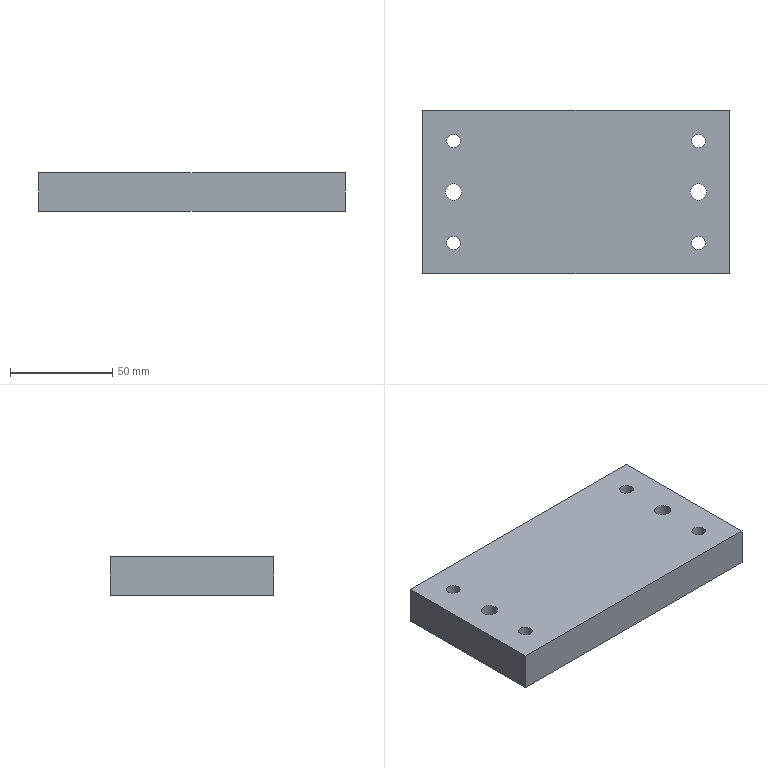Part | STEP file | SN10_010_005-01_PLACA | 1 solid | 12 faces | box 150 x 80 x 19 mm | volume 223453 mm3 | cylinder 6 | plane 6 | commonest cylinder face diameters 6.647 x4 8 x2
STEP:
#1=CARTESIAN_POINT('',(0.,0.,0.));
#2=DIRECTION('',(0.,0.,1.));
#3=DIRECTION('',(1.,0.,0.));
#4=AXIS2_PLACEMENT_3D('',#1,#2,#3);
#5=CARTESIAN_POINT('',(-57.083,-286.593,339.));
#6=VERTEX_POINT('',#5);
#7=CARTESIAN_POINT('',(-60.,-285.,339.));
#8=DIRECTION('',(0.,0.,-1.));
#9=DIRECTION('',(1.,0.,0.));
#10=AXIS2_PLACEMENT_3D('',#7,#8,#9);
#11=CIRCLE('',#10,3.324);
#12=CARTESIAN_POINT('',(-60.,-285.,338.9));
#13=DIRECTION('',(0.,0.,-1.));
#14=DIRECTION('',(0.8776,-0.4794,0.));
#15=AXIS2_PLACEMENT_3D('',#12,#13,#14);
#16=CYLINDRICAL_SURFACE('',#15,3.324);
#17=CARTESIAN_POINT('',(-0.5,-0.1));
#18=DIRECTION('',(1.,0.));
#19=VECTOR('',#18,1.);
#20=LINE('',#17,#19);
#21=(GEOMETRIC_REPRESENTATION_CONTEXT(2)PARAMETRIC_REPRESENTATION_CONTEXT()REPRESENTATION_CONTEXT('',''));
#22=DEFINITIONAL_REPRESENTATION('',(#20),#21);
#23=PCURVE('',#16,#22);
#24=CARTESIAN_POINT('',(0.,0.,339.));
#25=DIRECTION('',(0.,0.,1.));
#26=DIRECTION('',(1.,0.,0.));
#27=AXIS2_PLACEMENT_3D('',#24,#25,#26);
#28=PLANE('',#27);
#29=CARTESIAN_POINT('',(-56.676,-285.));
#30=CARTESIAN_POINT('',(-56.676,-290.756));
#31=CARTESIAN_POINT('',(-61.662,-287.878));
#32=CARTESIAN_POINT('',(-66.647,-285.));
#33=CARTESIAN_POINT('',(-61.662,-282.122));
#34=CARTESIAN_POINT('',(-56.676,-279.244));
#35=CARTESIAN_POINT('',(-56.676,-285.));
#36=(BOUNDED_CURVE()B_SPLINE_CURVE(2,(#29,#30,#31,#32,#33,#34,#35),.UNSPECIFIED.,.T.,.F.)B_SPLINE_CURVE_WITH_KNOTS((1,2,2,2,2,1),(-2.094,0.,2.094,4.189,6.283,8.378),.UNSPECIFIED.)CURVE()GEOMETRIC_REPRESENTATION_ITEM()RATIONAL_B_SPLINE_CURVE((1.,0.5,1.,0.5,1.,0.5,1.))REPRESENTATION_ITEM(''));
#37=(GEOMETRIC_REPRESENTATION_CONTEXT(2)PARAMETRIC_REPRESENTATION_CONTEXT()REPRESENTATION_CONTEXT('',''));
#38=DEFINITIONAL_REPRESENTATION('',(#36),#37);
#39=PCURVE('',#28,#38);
#40=SURFACE_CURVE('',#11,(#23,#39),.PCURVE_S1.);
#41=EDGE_CURVE('',#6,#6,#40,.T.);
#42=ORIENTED_EDGE('',*,*,#41,.T.);
#43=CARTESIAN_POINT('',(-57.083,-286.593,320.));
#44=VERTEX_POINT('',#43);
#45=CARTESIAN_POINT('',(-57.083,-286.593,339.));
#46=CARTESIAN_POINT('',(-57.083,-286.593,320.));
#47=B_SPLINE_CURVE_WITH_KNOTS('',1,(#45,#46),.UNSPECIFIED.,.F.,.F.,(2,2),(-0.1,18.9),.PIECEWISE_BEZIER_KNOTS.);
#48=CARTESIAN_POINT('',(6.283,0.));
#49=DIRECTION('',(0.,1.));
#50=VECTOR('',#49,1.);
#51=LINE('',#48,#50);
#52=(GEOMETRIC_REPRESENTATION_CONTEXT(2)PARAMETRIC_REPRESENTATION_CONTEXT()REPRESENTATION_CONTEXT('',''));
#53=DEFINITIONAL_REPRESENTATION('',(#51),#52);
#54=PCURVE('',#16,#53);
#55=CARTESIAN_POINT('',(0.,0.));
#56=DIRECTION('',(0.,1.));
#57=VECTOR('',#56,1.);
#58=LINE('',#55,#57);
#59=(GEOMETRIC_REPRESENTATION_CONTEXT(2)PARAMETRIC_REPRESENTATION_CONTEXT()REPRESENTATION_CONTEXT('',''));
#60=DEFINITIONAL_REPRESENTATION('',(#58),#59);
#61=PCURVE('',#16,#60);
#62=SEAM_CURVE('',#47,(#54,#61),.PCURVE_S1.);
#63=EDGE_CURVE('',#6,#44,#62,.T.);
#64=ORIENTED_EDGE('',*,*,#63,.T.);
#65=CARTESIAN_POINT('',(-60.,-285.,320.));
#66=DIRECTION('',(0.,0.,-1.));
#67=DIRECTION('',(1.,0.,0.));
#68=AXIS2_PLACEMENT_3D('',#65,#66,#67);
#69=CIRCLE('',#68,3.324);
#70=CARTESIAN_POINT('',(-0.5,18.9));
#71=DIRECTION('',(1.,0.));
#72=VECTOR('',#71,1.);
#73=LINE('',#70,#72);
#74=(GEOMETRIC_REPRESENTATION_CONTEXT(2)PARAMETRIC_REPRESENTATION_CONTEXT()REPRESENTATION_CONTEXT('',''));
#75=DEFINITIONAL_REPRESENTATION('',(#73),#74);
#76=PCURVE('',#16,#75);
#77=CARTESIAN_POINT('',(0.,0.,320.));
#78=DIRECTION('',(0.,0.,1.));
#79=DIRECTION('',(1.,0.,0.));
#80=AXIS2_PLACEMENT_3D('',#77,#78,#79);
#81=PLANE('',#80);
#82=CARTESIAN_POINT('',(-56.676,-285.));
#83=CARTESIAN_POINT('',(-56.676,-290.756));
#84=CARTESIAN_POINT('',(-61.662,-287.878));
#85=CARTESIAN_POINT('',(-66.647,-285.));
#86=CARTESIAN_POINT('',(-61.662,-282.122));
#87=CARTESIAN_POINT('',(-56.676,-279.244));
#88=CARTESIAN_POINT('',(-56.676,-285.));
#89=(BOUNDED_CURVE()B_SPLINE_CURVE(2,(#82,#83,#84,#85,#86,#87,#88),.UNSPECIFIED.,.T.,.F.)B_SPLINE_CURVE_WITH_KNOTS((1,2,2,2,2,1),(-2.094,0.,2.094,4.189,6.283,8.378),.UNSPECIFIED.)CURVE()GEOMETRIC_REPRESENTATION_ITEM()RATIONAL_B_SPLINE_CURVE((1.,0.5,1.,0.5,1.,0.5,1.))REPRESENTATION_ITEM(''));
#90=(GEOMETRIC_REPRESENTATION_CONTEXT(2)PARAMETRIC_REPRESENTATION_CONTEXT()REPRESENTATION_CONTEXT('',''));
#91=DEFINITIONAL_REPRESENTATION('',(#89),#90);
#92=PCURVE('',#81,#91);
#93=SURFACE_CURVE('',#69,(#76,#92),.PCURVE_S1.);
#94=EDGE_CURVE('',#44,#44,#93,.T.);
#95=ORIENTED_EDGE('',*,*,#94,.F.);
#96=ORIENTED_EDGE('',*,*,#63,.F.);
#97=EDGE_LOOP('',(#42,#64,#95,#96));
#98=FACE_BOUND('',#97,.F.);
#99=ADVANCED_FACE('',(#98),#16,.F.);
#100=CARTESIAN_POINT('',(-75.,-270.,320.));
#101=VERTEX_POINT('',#100);
#102=CARTESIAN_POINT('',(-75.,-270.,339.));
#103=VERTEX_POINT('',#102);
#104=CARTESIAN_POINT('',(-75.,-270.,320.));
#105=DIRECTION('',(0.,0.,1.));
#106=VECTOR('',#105,1.);
#107=LINE('',#104,#106);
#108=CARTESIAN_POINT('',(-75.,-270.,320.));
#109=DIRECTION('',(-1.,0.,0.));
#110=DIRECTION('',(0.,0.,1.));
#111=AXIS2_PLACEMENT_3D('',#108,#109,#110);
#112=PLANE('',#111);
#113=CARTESIAN_POINT('',(0.,0.));
#114=DIRECTION('',(1.,0.));
#115=VECTOR('',#114,1.);
#116=LINE('',#113,#115);
#117=(GEOMETRIC_REPRESENTATION_CONTEXT(2)PARAMETRIC_REPRESENTATION_CONTEXT()REPRESENTATION_CONTEXT('',''));
#118=DEFINITIONAL_REPRESENTATION('',(#116),#117);
#119=PCURVE('',#112,#118);
#120=CARTESIAN_POINT('',(-75.,-270.,320.));
#121=DIRECTION('',(0.,-1.,0.));
#122=DIRECTION('',(0.,0.,-1.));
#123=AXIS2_PLACEMENT_3D('',#120,#121,#122);
#124=PLANE('',#123);
#125=CARTESIAN_POINT('',(0.,0.));
#126=DIRECTION('',(-1.,0.));
#127=VECTOR('',#126,1.);
#128=LINE('',#125,#127);
#129=(GEOMETRIC_REPRESENTATION_CONTEXT(2)PARAMETRIC_REPRESENTATION_CONTEXT()REPRESENTATION_CONTEXT('',''));
#130=DEFINITIONAL_REPRESENTATION('',(#128),#129);
#131=PCURVE('',#124,#130);
#132=SURFACE_CURVE('',#107,(#119,#131),.PCURVE_S1.);
#133=EDGE_CURVE('',#101,#103,#132,.T.);
#134=ORIENTED_EDGE('',*,*,#133,.F.);
#135=CARTESIAN_POINT('',(-75.,-350.,320.));
#136=VERTEX_POINT('',#135);
#137=CARTESIAN_POINT('',(-75.,-270.,320.));
#138=DIRECTION('',(0.,-1.,0.));
#139=VECTOR('',#138,1.);
#140=LINE('',#137,#139);
#141=CARTESIAN_POINT('',(0.,0.));
#142=DIRECTION('',(0.,-1.));
#143=VECTOR('',#142,1.);
#144=LINE('',#141,#143);
#145=(GEOMETRIC_REPRESENTATION_CONTEXT(2)PARAMETRIC_REPRESENTATION_CONTEXT()REPRESENTATION_CONTEXT('',''));
#146=DEFINITIONAL_REPRESENTATION('',(#144),#145);
#147=PCURVE('',#112,#146);
#148=CARTESIAN_POINT('',(-75.,-270.));
#149=DIRECTION('',(0.,-1.));
#150=VECTOR('',#149,1.);
#151=LINE('',#148,#150);
#152=(GEOMETRIC_REPRESENTATION_CONTEXT(2)PARAMETRIC_REPRESENTATION_CONTEXT()REPRESENTATION_CONTEXT('',''));
#153=DEFINITIONAL_REPRESENTATION('',(#151),#152);
#154=PCURVE('',#81,#153);
#155=SURFACE_CURVE('',#140,(#147,#154),.PCURVE_S1.);
#156=EDGE_CURVE('',#101,#136,#155,.T.);
#157=ORIENTED_EDGE('',*,*,#156,.T.);
#158=CARTESIAN_POINT('',(-75.,-350.,339.));
#159=VERTEX_POINT('',#158);
#160=CARTESIAN_POINT('',(-75.,-350.,320.));
#161=DIRECTION('',(0.,0.,1.));
#162=VECTOR('',#161,1.);
#163=LINE('',#160,#162);
#164=CARTESIAN_POINT('',(0.,-80.));
#165=DIRECTION('',(1.,0.));
#166=VECTOR('',#165,1.);
#167=LINE('',#164,#166);
#168=(GEOMETRIC_REPRESENTATION_CONTEXT(2)PARAMETRIC_REPRESENTATION_CONTEXT()REPRESENTATION_CONTEXT('',''));
#169=DEFINITIONAL_REPRESENTATION('',(#167),#168);
#170=PCURVE('',#112,#169);
#171=CARTESIAN_POINT('',(75.,-350.,320.));
#172=DIRECTION('',(0.,1.,0.));
#173=DIRECTION('',(0.,0.,1.));
#174=AXIS2_PLACEMENT_3D('',#171,#172,#173);
#175=PLANE('',#174);
#176=CARTESIAN_POINT('',(0.,-150.));
#177=DIRECTION('',(1.,0.));
#178=VECTOR('',#177,1.);
#179=LINE('',#176,#178);
#180=(GEOMETRIC_REPRESENTATION_CONTEXT(2)PARAMETRIC_REPRESENTATION_CONTEXT()REPRESENTATION_CONTEXT('',''));
#181=DEFINITIONAL_REPRESENTATION('',(#179),#180);
#182=PCURVE('',#175,#181);
#183=SURFACE_CURVE('',#163,(#170,#182),.PCURVE_S1.);
#184=EDGE_CURVE('',#136,#159,#183,.T.);
#185=ORIENTED_EDGE('',*,*,#184,.T.);
#186=CARTESIAN_POINT('',(-75.,-270.,339.));
#187=DIRECTION('',(0.,-1.,0.));
#188=VECTOR('',#187,1.);
#189=LINE('',#186,#188);
#190=CARTESIAN_POINT('',(19.,0.));
#191=DIRECTION('',(0.,-1.));
#192=VECTOR('',#191,1.);
#193=LINE('',#190,#192);
#194=(GEOMETRIC_REPRESENTATION_CONTEXT(2)PARAMETRIC_REPRESENTATION_CONTEXT()REPRESENTATION_CONTEXT('',''));
#195=DEFINITIONAL_REPRESENTATION('',(#193),#194);
#196=PCURVE('',#112,#195);
#197=CARTESIAN_POINT('',(-75.,-270.));
#198=DIRECTION('',(0.,-1.));
#199=VECTOR('',#198,1.);
#200=LINE('',#197,#199);
#201=(GEOMETRIC_REPRESENTATION_CONTEXT(2)PARAMETRIC_REPRESENTATION_CONTEXT()REPRESENTATION_CONTEXT('',''));
#202=DEFINITIONAL_REPRESENTATION('',(#200),#201);
#203=PCURVE('',#28,#202);
#204=SURFACE_CURVE('',#189,(#196,#203),.PCURVE_S1.);
#205=EDGE_CURVE('',#103,#159,#204,.T.);
#206=ORIENTED_EDGE('',*,*,#205,.F.);
#207=EDGE_LOOP('',(#134,#157,#185,#206));
#208=FACE_BOUND('',#207,.T.);
#209=ADVANCED_FACE('',(#208),#112,.T.);
#210=ORIENTED_EDGE('',*,*,#184,.F.);
#211=CARTESIAN_POINT('',(75.,-350.,320.));
#212=VERTEX_POINT('',#211);
#213=CARTESIAN_POINT('',(75.,-350.,320.));
#214=DIRECTION('',(-1.,0.,0.));
#215=VECTOR('',#214,1.);
#216=LINE('',#213,#215);
#217=CARTESIAN_POINT('',(0.,0.));
#218=DIRECTION('',(0.,-1.));
#219=VECTOR('',#218,1.);
#220=LINE('',#217,#219);
#221=(GEOMETRIC_REPRESENTATION_CONTEXT(2)PARAMETRIC_REPRESENTATION_CONTEXT()REPRESENTATION_CONTEXT('',''));
#222=DEFINITIONAL_REPRESENTATION('',(#220),#221);
#223=PCURVE('',#175,#222);
#224=CARTESIAN_POINT('',(75.,-350.));
#225=DIRECTION('',(-1.,0.));
#226=VECTOR('',#225,1.);
#227=LINE('',#224,#226);
#228=(GEOMETRIC_REPRESENTATION_CONTEXT(2)PARAMETRIC_REPRESENTATION_CONTEXT()REPRESENTATION_CONTEXT('',''));
#229=DEFINITIONAL_REPRESENTATION('',(#227),#228);
#230=PCURVE('',#81,#229);
#231=SURFACE_CURVE('',#216,(#223,#230),.PCURVE_S1.);
#232=EDGE_CURVE('',#212,#136,#231,.T.);
#233=ORIENTED_EDGE('',*,*,#232,.F.);
#234=CARTESIAN_POINT('',(75.,-350.,339.));
#235=VERTEX_POINT('',#234);
#236=CARTESIAN_POINT('',(75.,-350.,320.));
#237=DIRECTION('',(0.,0.,1.));
#238=VECTOR('',#237,1.);
#239=LINE('',#236,#238);
#240=CARTESIAN_POINT('',(0.,0.));
#241=DIRECTION('',(1.,0.));
#242=VECTOR('',#241,1.);
#243=LINE('',#240,#242);
#244=(GEOMETRIC_REPRESENTATION_CONTEXT(2)PARAMETRIC_REPRESENTATION_CONTEXT()REPRESENTATION_CONTEXT('',''));
#245=DEFINITIONAL_REPRESENTATION('',(#243),#244);
#246=PCURVE('',#175,#245);
#247=CARTESIAN_POINT('',(75.,-350.,320.));
#248=DIRECTION('',(1.,0.,0.));
#249=DIRECTION('',(0.,0.,-1.));
#250=AXIS2_PLACEMENT_3D('',#247,#248,#249);
#251=PLANE('',#250);
#252=CARTESIAN_POINT('',(0.,0.));
#253=DIRECTION('',(-1.,0.));
#254=VECTOR('',#253,1.);
#255=LINE('',#252,#254);
#256=(GEOMETRIC_REPRESENTATION_CONTEXT(2)PARAMETRIC_REPRESENTATION_CONTEXT()REPRESENTATION_CONTEXT('',''));
#257=DEFINITIONAL_REPRESENTATION('',(#255),#256);
#258=PCURVE('',#251,#257);
#259=SURFACE_CURVE('',#239,(#246,#258),.PCURVE_S1.);
#260=EDGE_CURVE('',#212,#235,#259,.T.);
#261=ORIENTED_EDGE('',*,*,#260,.T.);
#262=CARTESIAN_POINT('',(75.,-350.,339.));
#263=DIRECTION('',(-1.,0.,0.));
#264=VECTOR('',#263,1.);
#265=LINE('',#262,#264);
#266=CARTESIAN_POINT('',(19.,0.));
#267=DIRECTION('',(0.,-1.));
#268=VECTOR('',#267,1.);
#269=LINE('',#266,#268);
#270=(GEOMETRIC_REPRESENTATION_CONTEXT(2)PARAMETRIC_REPRESENTATION_CONTEXT()REPRESENTATION_CONTEXT('',''));
#271=DEFINITIONAL_REPRESENTATION('',(#269),#270);
#272=PCURVE('',#175,#271);
#273=CARTESIAN_POINT('',(75.,-350.));
#274=DIRECTION('',(-1.,0.));
#275=VECTOR('',#274,1.);
#276=LINE('',#273,#275);
#277=(GEOMETRIC_REPRESENTATION_CONTEXT(2)PARAMETRIC_REPRESENTATION_CONTEXT()REPRESENTATION_CONTEXT('',''));
#278=DEFINITIONAL_REPRESENTATION('',(#276),#277);
#279=PCURVE('',#28,#278);
#280=SURFACE_CURVE('',#265,(#272,#279),.PCURVE_S1.);
#281=EDGE_CURVE('',#235,#159,#280,.T.);
#282=ORIENTED_EDGE('',*,*,#281,.T.);
#283=EDGE_LOOP('',(#210,#233,#261,#282));
#284=FACE_BOUND('',#283,.T.);
#285=ADVANCED_FACE('',(#284),#175,.F.);
#286=ORIENTED_EDGE('',*,*,#260,.F.);
#287=CARTESIAN_POINT('',(75.,-270.,320.));
#288=VERTEX_POINT('',#287);
#289=CARTESIAN_POINT('',(75.,-350.,320.));
#290=DIRECTION('',(0.,1.,0.));
#291=VECTOR('',#290,1.);
#292=LINE('',#289,#291);
#293=CARTESIAN_POINT('',(0.,0.));
#294=DIRECTION('',(0.,1.));
#295=VECTOR('',#294,1.);
#296=LINE('',#293,#295);
#297=(GEOMETRIC_REPRESENTATION_CONTEXT(2)PARAMETRIC_REPRESENTATION_CONTEXT()REPRESENTATION_CONTEXT('',''));
#298=DEFINITIONAL_REPRESENTATION('',(#296),#297);
#299=PCURVE('',#251,#298);
#300=CARTESIAN_POINT('',(75.,-350.));
#301=DIRECTION('',(0.,1.));
#302=VECTOR('',#301,1.);
#303=LINE('',#300,#302);
#304=(GEOMETRIC_REPRESENTATION_CONTEXT(2)PARAMETRIC_REPRESENTATION_CONTEXT()REPRESENTATION_CONTEXT('',''));
#305=DEFINITIONAL_REPRESENTATION('',(#303),#304);
#306=PCURVE('',#81,#305);
#307=SURFACE_CURVE('',#292,(#299,#306),.PCURVE_S1.);
#308=EDGE_CURVE('',#212,#288,#307,.T.);
#309=ORIENTED_EDGE('',*,*,#308,.T.);
#310=CARTESIAN_POINT('',(75.,-270.,339.));
#311=VERTEX_POINT('',#310);
#312=CARTESIAN_POINT('',(75.,-270.,320.));
#313=DIRECTION('',(0.,0.,1.));
#314=VECTOR('',#313,1.);
#315=LINE('',#312,#314);
#316=CARTESIAN_POINT('',(0.,80.));
#317=DIRECTION('',(-1.,0.));
#318=VECTOR('',#317,1.);
#319=LINE('',#316,#318);
#320=(GEOMETRIC_REPRESENTATION_CONTEXT(2)PARAMETRIC_REPRESENTATION_CONTEXT()REPRESENTATION_CONTEXT('',''));
#321=DEFINITIONAL_REPRESENTATION('',(#319),#320);
#322=PCURVE('',#251,#321);
#323=CARTESIAN_POINT('',(0.,150.));
#324=DIRECTION('',(-1.,0.));
#325=VECTOR('',#324,1.);
#326=LINE('',#323,#325);
#327=(GEOMETRIC_REPRESENTATION_CONTEXT(2)PARAMETRIC_REPRESENTATION_CONTEXT()REPRESENTATION_CONTEXT('',''));
#328=DEFINITIONAL_REPRESENTATION('',(#326),#327);
#329=PCURVE('',#124,#328);
#330=SURFACE_CURVE('',#315,(#322,#329),.PCURVE_S1.);
#331=EDGE_CURVE('',#288,#311,#330,.T.);
#332=ORIENTED_EDGE('',*,*,#331,.T.);
#333=CARTESIAN_POINT('',(75.,-350.,339.));
#334=DIRECTION('',(0.,1.,0.));
#335=VECTOR('',#334,1.);
#336=LINE('',#333,#335);
#337=CARTESIAN_POINT('',(-19.,0.));
#338=DIRECTION('',(0.,1.));
#339=VECTOR('',#338,1.);
#340=LINE('',#337,#339);
#341=(GEOMETRIC_REPRESENTATION_CONTEXT(2)PARAMETRIC_REPRESENTATION_CONTEXT()REPRESENTATION_CONTEXT('',''));
#342=DEFINITIONAL_REPRESENTATION('',(#340),#341);
#343=PCURVE('',#251,#342);
#344=CARTESIAN_POINT('',(75.,-350.));
#345=DIRECTION('',(0.,1.));
#346=VECTOR('',#345,1.);
#347=LINE('',#344,#346);
#348=(GEOMETRIC_REPRESENTATION_CONTEXT(2)PARAMETRIC_REPRESENTATION_CONTEXT()REPRESENTATION_CONTEXT('',''));
#349=DEFINITIONAL_REPRESENTATION('',(#347),#348);
#350=PCURVE('',#28,#349);
#351=SURFACE_CURVE('',#336,(#343,#350),.PCURVE_S1.);
#352=EDGE_CURVE('',#235,#311,#351,.T.);
#353=ORIENTED_EDGE('',*,*,#352,.F.);
#354=EDGE_LOOP('',(#286,#309,#332,#353));
#355=FACE_BOUND('',#354,.T.);
#356=ADVANCED_FACE('',(#355),#251,.T.);
#357=ORIENTED_EDGE('',*,*,#331,.F.);
#358=CARTESIAN_POINT('',(-75.,-270.,320.));
#359=DIRECTION('',(1.,0.,0.));
#360=VECTOR('',#359,1.);
#361=LINE('',#358,#360);
#362=CARTESIAN_POINT('',(0.,0.));
#363=DIRECTION('',(0.,1.));
#364=VECTOR('',#363,1.);
#365=LINE('',#362,#364);
#366=(GEOMETRIC_REPRESENTATION_CONTEXT(2)PARAMETRIC_REPRESENTATION_CONTEXT()REPRESENTATION_CONTEXT('',''));
#367=DEFINITIONAL_REPRESENTATION('',(#365),#366);
#368=PCURVE('',#124,#367);
#369=CARTESIAN_POINT('',(-75.,-270.));
#370=DIRECTION('',(1.,0.));
#371=VECTOR('',#370,1.);
#372=LINE('',#369,#371);
#373=(GEOMETRIC_REPRESENTATION_CONTEXT(2)PARAMETRIC_REPRESENTATION_CONTEXT()REPRESENTATION_CONTEXT('',''));
#374=DEFINITIONAL_REPRESENTATION('',(#372),#373);
#375=PCURVE('',#81,#374);
#376=SURFACE_CURVE('',#361,(#368,#375),.PCURVE_S1.);
#377=EDGE_CURVE('',#101,#288,#376,.T.);
#378=ORIENTED_EDGE('',*,*,#377,.F.);
#379=ORIENTED_EDGE('',*,*,#133,.T.);
#380=CARTESIAN_POINT('',(-75.,-270.,339.));
#381=DIRECTION('',(1.,0.,0.));
#382=VECTOR('',#381,1.);
#383=LINE('',#380,#382);
#384=CARTESIAN_POINT('',(-19.,0.));
#385=DIRECTION('',(0.,1.));
#386=VECTOR('',#385,1.);
#387=LINE('',#384,#386);
#388=(GEOMETRIC_REPRESENTATION_CONTEXT(2)PARAMETRIC_REPRESENTATION_CONTEXT()REPRESENTATION_CONTEXT('',''));
#389=DEFINITIONAL_REPRESENTATION('',(#387),#388);
#390=PCURVE('',#124,#389);
#391=CARTESIAN_POINT('',(-75.,-270.));
#392=DIRECTION('',(1.,0.));
#393=VECTOR('',#392,1.);
#394=LINE('',#391,#393);
#395=(GEOMETRIC_REPRESENTATION_CONTEXT(2)PARAMETRIC_REPRESENTATION_CONTEXT()REPRESENTATION_CONTEXT('',''));
#396=DEFINITIONAL_REPRESENTATION('',(#394),#395);
#397=PCURVE('',#28,#396);
#398=SURFACE_CURVE('',#383,(#390,#397),.PCURVE_S1.);
#399=EDGE_CURVE('',#103,#311,#398,.T.);
#400=ORIENTED_EDGE('',*,*,#399,.T.);
#401=EDGE_LOOP('',(#357,#378,#379,#400));
#402=FACE_BOUND('',#401,.T.);
#403=ADVANCED_FACE('',(#402),#124,.F.);
#404=CARTESIAN_POINT('',(-56.49,-311.918,339.));
#405=VERTEX_POINT('',#404);
#406=CARTESIAN_POINT('',(-60.,-310.,339.));
#407=DIRECTION('',(0.,0.,-1.));
#408=DIRECTION('',(1.,0.,0.));
#409=AXIS2_PLACEMENT_3D('',#406,#407,#408);
#410=CIRCLE('',#409,4.);
#411=CARTESIAN_POINT('',(-60.,-310.,338.9));
#412=DIRECTION('',(0.,0.,-1.));
#413=DIRECTION('',(0.8776,-0.4794,0.));
#414=AXIS2_PLACEMENT_3D('',#411,#412,#413);
#415=CYLINDRICAL_SURFACE('',#414,4.);
#416=CARTESIAN_POINT('',(-0.5,-0.1));
#417=DIRECTION('',(1.,0.));
#418=VECTOR('',#417,1.);
#419=LINE('',#416,#418);
#420=(GEOMETRIC_REPRESENTATION_CONTEXT(2)PARAMETRIC_REPRESENTATION_CONTEXT()REPRESENTATION_CONTEXT('',''));
#421=DEFINITIONAL_REPRESENTATION('',(#419),#420);
#422=PCURVE('',#415,#421);
#423=CARTESIAN_POINT('',(-56.,-310.));
#424=CARTESIAN_POINT('',(-56.,-316.928));
#425=CARTESIAN_POINT('',(-62.,-313.464));
#426=CARTESIAN_POINT('',(-68.,-310.));
#427=CARTESIAN_POINT('',(-62.,-306.536));
#428=CARTESIAN_POINT('',(-56.,-303.072));
#429=CARTESIAN_POINT('',(-56.,-310.));
#430=(BOUNDED_CURVE()B_SPLINE_CURVE(2,(#423,#424,#425,#426,#427,#428,#429),.UNSPECIFIED.,.T.,.F.)B_SPLINE_CURVE_WITH_KNOTS((1,2,2,2,2,1),(-2.094,0.,2.094,4.189,6.283,8.378),.UNSPECIFIED.)CURVE()GEOMETRIC_REPRESENTATION_ITEM()RATIONAL_B_SPLINE_CURVE((1.,0.5,1.,0.5,1.,0.5,1.))REPRESENTATION_ITEM(''));
#431=(GEOMETRIC_REPRESENTATION_CONTEXT(2)PARAMETRIC_REPRESENTATION_CONTEXT()REPRESENTATION_CONTEXT('',''));
#432=DEFINITIONAL_REPRESENTATION('',(#430),#431);
#433=PCURVE('',#28,#432);
#434=SURFACE_CURVE('',#410,(#422,#433),.PCURVE_S1.);
#435=EDGE_CURVE('',#405,#405,#434,.T.);
#436=ORIENTED_EDGE('',*,*,#435,.T.);
#437=CARTESIAN_POINT('',(-56.49,-311.918,320.));
#438=VERTEX_POINT('',#437);
#439=CARTESIAN_POINT('',(-56.49,-311.918,339.));
#440=CARTESIAN_POINT('',(-56.49,-311.918,320.));
#441=B_SPLINE_CURVE_WITH_KNOTS('',1,(#439,#440),.UNSPECIFIED.,.F.,.F.,(2,2),(-0.1,18.9),.PIECEWISE_BEZIER_KNOTS.);
#442=CARTESIAN_POINT('',(6.283,0.));
#443=DIRECTION('',(0.,1.));
#444=VECTOR('',#443,1.);
#445=LINE('',#442,#444);
#446=(GEOMETRIC_REPRESENTATION_CONTEXT(2)PARAMETRIC_REPRESENTATION_CONTEXT()REPRESENTATION_CONTEXT('',''));
#447=DEFINITIONAL_REPRESENTATION('',(#445),#446);
#448=PCURVE('',#415,#447);
#449=CARTESIAN_POINT('',(0.,0.));
#450=DIRECTION('',(0.,1.));
#451=VECTOR('',#450,1.);
#452=LINE('',#449,#451);
#453=(GEOMETRIC_REPRESENTATION_CONTEXT(2)PARAMETRIC_REPRESENTATION_CONTEXT()REPRESENTATION_CONTEXT('',''));
#454=DEFINITIONAL_REPRESENTATION('',(#452),#453);
#455=PCURVE('',#415,#454);
#456=SEAM_CURVE('',#441,(#448,#455),.PCURVE_S1.);
#457=EDGE_CURVE('',#405,#438,#456,.T.);
#458=ORIENTED_EDGE('',*,*,#457,.T.);
#459=CARTESIAN_POINT('',(-60.,-310.,320.));
#460=DIRECTION('',(0.,0.,-1.));
#461=DIRECTION('',(1.,0.,0.));
#462=AXIS2_PLACEMENT_3D('',#459,#460,#461);
#463=CIRCLE('',#462,4.);
#464=CARTESIAN_POINT('',(-0.5,18.9));
#465=DIRECTION('',(1.,0.));
#466=VECTOR('',#465,1.);
#467=LINE('',#464,#466);
#468=(GEOMETRIC_REPRESENTATION_CONTEXT(2)PARAMETRIC_REPRESENTATION_CONTEXT()REPRESENTATION_CONTEXT('',''));
#469=DEFINITIONAL_REPRESENTATION('',(#467),#468);
#470=PCURVE('',#415,#469);
#471=CARTESIAN_POINT('',(-56.,-310.));
#472=CARTESIAN_POINT('',(-56.,-316.928));
#473=CARTESIAN_POINT('',(-62.,-313.464));
#474=CARTESIAN_POINT('',(-68.,-310.));
#475=CARTESIAN_POINT('',(-62.,-306.536));
#476=CARTESIAN_POINT('',(-56.,-303.072));
#477=CARTESIAN_POINT('',(-56.,-310.));
#478=(BOUNDED_CURVE()B_SPLINE_CURVE(2,(#471,#472,#473,#474,#475,#476,#477),.UNSPECIFIED.,.T.,.F.)B_SPLINE_CURVE_WITH_KNOTS((1,2,2,2,2,1),(-2.094,0.,2.094,4.189,6.283,8.378),.UNSPECIFIED.)CURVE()GEOMETRIC_REPRESENTATION_ITEM()RATIONAL_B_SPLINE_CURVE((1.,0.5,1.,0.5,1.,0.5,1.))REPRESENTATION_ITEM(''));
#479=(GEOMETRIC_REPRESENTATION_CONTEXT(2)PARAMETRIC_REPRESENTATION_CONTEXT()REPRESENTATION_CONTEXT('',''));
#480=DEFINITIONAL_REPRESENTATION('',(#478),#479);
#481=PCURVE('',#81,#480);
#482=SURFACE_CURVE('',#463,(#470,#481),.PCURVE_S1.);
#483=EDGE_CURVE('',#438,#438,#482,.T.);
#484=ORIENTED_EDGE('',*,*,#483,.F.);
#485=ORIENTED_EDGE('',*,*,#457,.F.);
#486=EDGE_LOOP('',(#436,#458,#484,#485));
#487=FACE_BOUND('',#486,.F.);
#488=ADVANCED_FACE('',(#487),#415,.F.);
#489=CARTESIAN_POINT('',(56.49,-308.082,339.));
#490=VERTEX_POINT('',#489);
#491=CARTESIAN_POINT('',(60.,-310.,339.));
#492=DIRECTION('',(0.,0.,-1.));
#493=DIRECTION('',(1.,0.,0.));
#494=AXIS2_PLACEMENT_3D('',#491,#492,#493);
#495=CIRCLE('',#494,4.);
#496=CARTESIAN_POINT('',(60.,-310.,338.9));
#497=DIRECTION('',(0.,0.,-1.));
#498=DIRECTION('',(0.8776,-0.4794,0.));
#499=AXIS2_PLACEMENT_3D('',#496,#497,#498);
#500=CYLINDRICAL_SURFACE('',#499,4.);
#501=CARTESIAN_POINT('',(-0.5,-0.1));
#502=DIRECTION('',(1.,0.));
#503=VECTOR('',#502,1.);
#504=LINE('',#501,#503);
#505=(GEOMETRIC_REPRESENTATION_CONTEXT(2)PARAMETRIC_REPRESENTATION_CONTEXT()REPRESENTATION_CONTEXT('',''));
#506=DEFINITIONAL_REPRESENTATION('',(#504),#505);
#507=PCURVE('',#500,#506);
#508=CARTESIAN_POINT('',(64.,-310.));
#509=CARTESIAN_POINT('',(64.,-316.928));
#510=CARTESIAN_POINT('',(58.,-313.464));
#511=CARTESIAN_POINT('',(52.,-310.));
#512=CARTESIAN_POINT('',(58.,-306.536));
#513=CARTESIAN_POINT('',(64.,-303.072));
#514=CARTESIAN_POINT('',(64.,-310.));
#515=(BOUNDED_CURVE()B_SPLINE_CURVE(2,(#508,#509,#510,#511,#512,#513,#514),.UNSPECIFIED.,.T.,.F.)B_SPLINE_CURVE_WITH_KNOTS((1,2,2,2,2,1),(-2.094,0.,2.094,4.189,6.283,8.378),.UNSPECIFIED.)CURVE()GEOMETRIC_REPRESENTATION_ITEM()RATIONAL_B_SPLINE_CURVE((1.,0.5,1.,0.5,1.,0.5,1.))REPRESENTATION_ITEM(''));
#516=(GEOMETRIC_REPRESENTATION_CONTEXT(2)PARAMETRIC_REPRESENTATION_CONTEXT()REPRESENTATION_CONTEXT('',''));
#517=DEFINITIONAL_REPRESENTATION('',(#515),#516);
#518=PCURVE('',#28,#517);
#519=SURFACE_CURVE('',#495,(#507,#518),.PCURVE_S1.);
#520=EDGE_CURVE('',#490,#490,#519,.T.);
#521=ORIENTED_EDGE('',*,*,#520,.T.);
#522=CARTESIAN_POINT('',(56.49,-308.082,320.));
#523=VERTEX_POINT('',#522);
#524=CARTESIAN_POINT('',(56.49,-308.082,339.));
#525=CARTESIAN_POINT('',(56.49,-308.082,320.));
#526=B_SPLINE_CURVE_WITH_KNOTS('',1,(#524,#525),.UNSPECIFIED.,.F.,.F.,(2,2),(-0.1,18.9),.PIECEWISE_BEZIER_KNOTS.);
#527=CARTESIAN_POINT('',(9.425,0.));
#528=DIRECTION('',(0.,1.));
#529=VECTOR('',#528,1.);
#530=LINE('',#527,#529);
#531=(GEOMETRIC_REPRESENTATION_CONTEXT(2)PARAMETRIC_REPRESENTATION_CONTEXT()REPRESENTATION_CONTEXT('',''));
#532=DEFINITIONAL_REPRESENTATION('',(#530),#531);
#533=PCURVE('',#500,#532);
#534=CARTESIAN_POINT('',(3.142,0.));
#535=DIRECTION('',(0.,1.));
#536=VECTOR('',#535,1.);
#537=LINE('',#534,#536);
#538=(GEOMETRIC_REPRESENTATION_CONTEXT(2)PARAMETRIC_REPRESENTATION_CONTEXT()REPRESENTATION_CONTEXT('',''));
#539=DEFINITIONAL_REPRESENTATION('',(#537),#538);
#540=PCURVE('',#500,#539);
#541=SEAM_CURVE('',#526,(#533,#540),.PCURVE_S1.);
#542=EDGE_CURVE('',#490,#523,#541,.T.);
#543=ORIENTED_EDGE('',*,*,#542,.T.);
#544=CARTESIAN_POINT('',(60.,-310.,320.));
#545=DIRECTION('',(0.,0.,-1.));
#546=DIRECTION('',(1.,0.,0.));
#547=AXIS2_PLACEMENT_3D('',#544,#545,#546);
#548=CIRCLE('',#547,4.);
#549=CARTESIAN_POINT('',(-0.5,18.9));
#550=DIRECTION('',(1.,0.));
#551=VECTOR('',#550,1.);
#552=LINE('',#549,#551);
#553=(GEOMETRIC_REPRESENTATION_CONTEXT(2)PARAMETRIC_REPRESENTATION_CONTEXT()REPRESENTATION_CONTEXT('',''));
#554=DEFINITIONAL_REPRESENTATION('',(#552),#553);
#555=PCURVE('',#500,#554);
#556=CARTESIAN_POINT('',(64.,-310.));
#557=CARTESIAN_POINT('',(64.,-316.928));
#558=CARTESIAN_POINT('',(58.,-313.464));
#559=CARTESIAN_POINT('',(52.,-310.));
#560=CARTESIAN_POINT('',(58.,-306.536));
#561=CARTESIAN_POINT('',(64.,-303.072));
#562=CARTESIAN_POINT('',(64.,-310.));
#563=(BOUNDED_CURVE()B_SPLINE_CURVE(2,(#556,#557,#558,#559,#560,#561,#562),.UNSPECIFIED.,.T.,.F.)B_SPLINE_CURVE_WITH_KNOTS((1,2,2,2,2,1),(-2.094,0.,2.094,4.189,6.283,8.378),.UNSPECIFIED.)CURVE()GEOMETRIC_REPRESENTATION_ITEM()RATIONAL_B_SPLINE_CURVE((1.,0.5,1.,0.5,1.,0.5,1.))REPRESENTATION_ITEM(''));
#564=(GEOMETRIC_REPRESENTATION_CONTEXT(2)PARAMETRIC_REPRESENTATION_CONTEXT()REPRESENTATION_CONTEXT('',''));
#565=DEFINITIONAL_REPRESENTATION('',(#563),#564);
#566=PCURVE('',#81,#565);
#567=SURFACE_CURVE('',#548,(#555,#566),.PCURVE_S1.);
#568=EDGE_CURVE('',#523,#523,#567,.T.);
#569=ORIENTED_EDGE('',*,*,#568,.F.);
#570=ORIENTED_EDGE('',*,*,#542,.F.);
#571=EDGE_LOOP('',(#521,#543,#569,#570));
#572=FACE_BOUND('',#571,.F.);
#573=ADVANCED_FACE('',(#572),#500,.F.);
#574=ORIENTED_EDGE('',*,*,#377,.T.);
#575=ORIENTED_EDGE('',*,*,#308,.F.);
#576=ORIENTED_EDGE('',*,*,#232,.T.);
#577=ORIENTED_EDGE('',*,*,#156,.F.);
#578=EDGE_LOOP('',(#574,#575,#576,#577));
#579=FACE_BOUND('',#578,.T.);
#580=ORIENTED_EDGE('',*,*,#94,.F.);
#581=EDGE_LOOP('',(#580));
#582=FACE_BOUND('',#581,.T.);
#583=ORIENTED_EDGE('',*,*,#568,.F.);
#584=EDGE_LOOP('',(#583));
#585=FACE_BOUND('',#584,.T.);
#586=ORIENTED_EDGE('',*,*,#483,.F.);
#587=EDGE_LOOP('',(#586));
#588=FACE_BOUND('',#587,.T.);
#589=CARTESIAN_POINT('',(62.917,-286.593,320.));
#590=VERTEX_POINT('',#589);
#591=CARTESIAN_POINT('',(60.,-285.,320.));
#592=DIRECTION('',(0.,0.,1.));
#593=DIRECTION('',(1.,0.,0.));
#594=AXIS2_PLACEMENT_3D('',#591,#592,#593);
#595=CIRCLE('',#594,3.324);
#596=CARTESIAN_POINT('',(60.,-285.));
#597=DIRECTION('',(1.,0.));
#598=AXIS2_PLACEMENT_2D('',#596,#597);
#599=CIRCLE('',#598,3.324);
#600=(GEOMETRIC_REPRESENTATION_CONTEXT(2)PARAMETRIC_REPRESENTATION_CONTEXT()REPRESENTATION_CONTEXT('',''));
#601=DEFINITIONAL_REPRESENTATION('',(#599),#600);
#602=PCURVE('',#81,#601);
#603=CARTESIAN_POINT('',(60.,-285.,338.9));
#604=DIRECTION('',(0.,0.,-1.));
#605=DIRECTION('',(0.8776,-0.4794,0.));
#606=AXIS2_PLACEMENT_3D('',#603,#604,#605);
#607=CYLINDRICAL_SURFACE('',#606,3.324);
#608=CARTESIAN_POINT('',(12.066,18.9));
#609=DIRECTION('',(-1.,0.));
#610=VECTOR('',#609,1.);
#611=LINE('',#608,#610);
#612=(GEOMETRIC_REPRESENTATION_CONTEXT(2)PARAMETRIC_REPRESENTATION_CONTEXT()REPRESENTATION_CONTEXT('',''));
#613=DEFINITIONAL_REPRESENTATION('',(#611),#612);
#614=PCURVE('',#607,#613);
#615=SURFACE_CURVE('',#595,(#602,#614),.PCURVE_S1.);
#616=EDGE_CURVE('',#590,#590,#615,.T.);
#617=ORIENTED_EDGE('',*,*,#616,.T.);
#618=EDGE_LOOP('',(#617));
#619=FACE_BOUND('',#618,.T.);
#620=CARTESIAN_POINT('',(-57.083,-336.593,320.));
#621=VERTEX_POINT('',#620);
#622=CARTESIAN_POINT('',(-60.,-335.,320.));
#623=DIRECTION('',(0.,0.,1.));
#624=DIRECTION('',(1.,0.,0.));
#625=AXIS2_PLACEMENT_3D('',#622,#623,#624);
#626=CIRCLE('',#625,3.324);
#627=CARTESIAN_POINT('',(-60.,-335.));
#628=DIRECTION('',(1.,0.));
#629=AXIS2_PLACEMENT_2D('',#627,#628);
#630=CIRCLE('',#629,3.324);
#631=(GEOMETRIC_REPRESENTATION_CONTEXT(2)PARAMETRIC_REPRESENTATION_CONTEXT()REPRESENTATION_CONTEXT('',''));
#632=DEFINITIONAL_REPRESENTATION('',(#630),#631);
#633=PCURVE('',#81,#632);
#634=CARTESIAN_POINT('',(-60.,-335.,338.9));
#635=DIRECTION('',(0.,0.,-1.));
#636=DIRECTION('',(0.8776,-0.4794,0.));
#637=AXIS2_PLACEMENT_3D('',#634,#635,#636);
#638=CYLINDRICAL_SURFACE('',#637,3.324);
#639=CARTESIAN_POINT('',(12.066,18.9));
#640=DIRECTION('',(-1.,0.));
#641=VECTOR('',#640,1.);
#642=LINE('',#639,#641);
#643=(GEOMETRIC_REPRESENTATION_CONTEXT(2)PARAMETRIC_REPRESENTATION_CONTEXT()REPRESENTATION_CONTEXT('',''));
#644=DEFINITIONAL_REPRESENTATION('',(#642),#643);
#645=PCURVE('',#638,#644);
#646=SURFACE_CURVE('',#626,(#633,#645),.PCURVE_S1.);
#647=EDGE_CURVE('',#621,#621,#646,.T.);
#648=ORIENTED_EDGE('',*,*,#647,.T.);
#649=EDGE_LOOP('',(#648));
#650=FACE_BOUND('',#649,.T.);
#651=CARTESIAN_POINT('',(62.917,-336.593,320.));
#652=VERTEX_POINT('',#651);
#653=CARTESIAN_POINT('',(60.,-335.,320.));
#654=DIRECTION('',(0.,0.,1.));
#655=DIRECTION('',(1.,0.,0.));
#656=AXIS2_PLACEMENT_3D('',#653,#654,#655);
#657=CIRCLE('',#656,3.324);
#658=CARTESIAN_POINT('',(60.,-335.));
#659=DIRECTION('',(1.,0.));
#660=AXIS2_PLACEMENT_2D('',#658,#659);
#661=CIRCLE('',#660,3.324);
#662=(GEOMETRIC_REPRESENTATION_CONTEXT(2)PARAMETRIC_REPRESENTATION_CONTEXT()REPRESENTATION_CONTEXT('',''));
#663=DEFINITIONAL_REPRESENTATION('',(#661),#662);
#664=PCURVE('',#81,#663);
#665=CARTESIAN_POINT('',(60.,-335.,338.9));
#666=DIRECTION('',(0.,0.,-1.));
#667=DIRECTION('',(0.8776,-0.4794,0.));
#668=AXIS2_PLACEMENT_3D('',#665,#666,#667);
#669=CYLINDRICAL_SURFACE('',#668,3.324);
#670=CARTESIAN_POINT('',(12.066,18.9));
#671=DIRECTION('',(-1.,0.));
#672=VECTOR('',#671,1.);
#673=LINE('',#670,#672);
#674=(GEOMETRIC_REPRESENTATION_CONTEXT(2)PARAMETRIC_REPRESENTATION_CONTEXT()REPRESENTATION_CONTEXT('',''));
#675=DEFINITIONAL_REPRESENTATION('',(#673),#674);
#676=PCURVE('',#669,#675);
#677=SURFACE_CURVE('',#657,(#664,#676),.PCURVE_S1.);
#678=EDGE_CURVE('',#652,#652,#677,.T.);
#679=ORIENTED_EDGE('',*,*,#678,.T.);
#680=EDGE_LOOP('',(#679));
#681=FACE_BOUND('',#680,.T.);
#682=ADVANCED_FACE('',(#579,#582,#585,#588,#619,#650,#681),#81,.F.);
#683=ORIENTED_EDGE('',*,*,#205,.T.);
#684=ORIENTED_EDGE('',*,*,#281,.F.);
#685=ORIENTED_EDGE('',*,*,#352,.T.);
#686=ORIENTED_EDGE('',*,*,#399,.F.);
#687=EDGE_LOOP('',(#683,#684,#685,#686));
#688=FACE_BOUND('',#687,.T.);
#689=ORIENTED_EDGE('',*,*,#41,.T.);
#690=EDGE_LOOP('',(#689));
#691=FACE_BOUND('',#690,.T.);
#692=ORIENTED_EDGE('',*,*,#520,.T.);
#693=EDGE_LOOP('',(#692));
#694=FACE_BOUND('',#693,.T.);
#695=ORIENTED_EDGE('',*,*,#435,.T.);
#696=EDGE_LOOP('',(#695));
#697=FACE_BOUND('',#696,.T.);
#698=CARTESIAN_POINT('',(62.917,-286.593,339.));
#699=VERTEX_POINT('',#698);
#700=CARTESIAN_POINT('',(60.,-285.,339.));
#701=DIRECTION('',(0.,0.,1.));
#702=DIRECTION('',(1.,0.,0.));
#703=AXIS2_PLACEMENT_3D('',#700,#701,#702);
#704=CIRCLE('',#703,3.324);
#705=CARTESIAN_POINT('',(60.,-285.));
#706=DIRECTION('',(1.,0.));
#707=AXIS2_PLACEMENT_2D('',#705,#706);
#708=CIRCLE('',#707,3.324);
#709=(GEOMETRIC_REPRESENTATION_CONTEXT(2)PARAMETRIC_REPRESENTATION_CONTEXT()REPRESENTATION_CONTEXT('',''));
#710=DEFINITIONAL_REPRESENTATION('',(#708),#709);
#711=PCURVE('',#28,#710);
#712=CARTESIAN_POINT('',(12.066,-0.1));
#713=DIRECTION('',(-1.,0.));
#714=VECTOR('',#713,1.);
#715=LINE('',#712,#714);
#716=(GEOMETRIC_REPRESENTATION_CONTEXT(2)PARAMETRIC_REPRESENTATION_CONTEXT()REPRESENTATION_CONTEXT('',''));
#717=DEFINITIONAL_REPRESENTATION('',(#715),#716);
#718=PCURVE('',#607,#717);
#719=SURFACE_CURVE('',#704,(#711,#718),.PCURVE_S1.);
#720=EDGE_CURVE('',#699,#699,#719,.T.);
#721=ORIENTED_EDGE('',*,*,#720,.F.);
#722=EDGE_LOOP('',(#721));
#723=FACE_BOUND('',#722,.T.);
#724=CARTESIAN_POINT('',(-57.083,-336.593,339.));
#725=VERTEX_POINT('',#724);
#726=CARTESIAN_POINT('',(-60.,-335.,339.));
#727=DIRECTION('',(0.,0.,1.));
#728=DIRECTION('',(1.,0.,0.));
#729=AXIS2_PLACEMENT_3D('',#726,#727,#728);
#730=CIRCLE('',#729,3.324);
#731=CARTESIAN_POINT('',(-60.,-335.));
#732=DIRECTION('',(1.,0.));
#733=AXIS2_PLACEMENT_2D('',#731,#732);
#734=CIRCLE('',#733,3.324);
#735=(GEOMETRIC_REPRESENTATION_CONTEXT(2)PARAMETRIC_REPRESENTATION_CONTEXT()REPRESENTATION_CONTEXT('',''));
#736=DEFINITIONAL_REPRESENTATION('',(#734),#735);
#737=PCURVE('',#28,#736);
#738=CARTESIAN_POINT('',(12.066,-0.1));
#739=DIRECTION('',(-1.,0.));
#740=VECTOR('',#739,1.);
#741=LINE('',#738,#740);
#742=(GEOMETRIC_REPRESENTATION_CONTEXT(2)PARAMETRIC_REPRESENTATION_CONTEXT()REPRESENTATION_CONTEXT('',''));
#743=DEFINITIONAL_REPRESENTATION('',(#741),#742);
#744=PCURVE('',#638,#743);
#745=SURFACE_CURVE('',#730,(#737,#744),.PCURVE_S1.);
#746=EDGE_CURVE('',#725,#725,#745,.T.);
#747=ORIENTED_EDGE('',*,*,#746,.F.);
#748=EDGE_LOOP('',(#747));
#749=FACE_BOUND('',#748,.T.);
#750=CARTESIAN_POINT('',(62.917,-336.593,339.));
#751=VERTEX_POINT('',#750);
#752=CARTESIAN_POINT('',(60.,-335.,339.));
#753=DIRECTION('',(0.,0.,1.));
#754=DIRECTION('',(1.,0.,0.));
#755=AXIS2_PLACEMENT_3D('',#752,#753,#754);
#756=CIRCLE('',#755,3.324);
#757=CARTESIAN_POINT('',(60.,-335.));
#758=DIRECTION('',(1.,0.));
#759=AXIS2_PLACEMENT_2D('',#757,#758);
#760=CIRCLE('',#759,3.324);
#761=(GEOMETRIC_REPRESENTATION_CONTEXT(2)PARAMETRIC_REPRESENTATION_CONTEXT()REPRESENTATION_CONTEXT('',''));
#762=DEFINITIONAL_REPRESENTATION('',(#760),#761);
#763=PCURVE('',#28,#762);
#764=CARTESIAN_POINT('',(12.066,-0.1));
#765=DIRECTION('',(-1.,0.));
#766=VECTOR('',#765,1.);
#767=LINE('',#764,#766);
#768=(GEOMETRIC_REPRESENTATION_CONTEXT(2)PARAMETRIC_REPRESENTATION_CONTEXT()REPRESENTATION_CONTEXT('',''));
#769=DEFINITIONAL_REPRESENTATION('',(#767),#768);
#770=PCURVE('',#669,#769);
#771=SURFACE_CURVE('',#756,(#763,#770),.PCURVE_S1.);
#772=EDGE_CURVE('',#751,#751,#771,.T.);
#773=ORIENTED_EDGE('',*,*,#772,.F.);
#774=EDGE_LOOP('',(#773));
#775=FACE_BOUND('',#774,.T.);
#776=ADVANCED_FACE('',(#688,#691,#694,#697,#723,#749,#775),#28,.T.);
#777=ORIENTED_EDGE('',*,*,#772,.F.);
#778=CARTESIAN_POINT('',(62.917,-336.593,339.));
#779=CARTESIAN_POINT('',(62.917,-336.593,320.));
#780=B_SPLINE_CURVE_WITH_KNOTS('',1,(#778,#779),.UNSPECIFIED.,.F.,.F.,(2,2),(-0.1,18.9),.PIECEWISE_BEZIER_KNOTS.);
#781=CARTESIAN_POINT('',(6.283,0.));
#782=DIRECTION('',(0.,1.));
#783=VECTOR('',#782,1.);
#784=LINE('',#781,#783);
#785=(GEOMETRIC_REPRESENTATION_CONTEXT(2)PARAMETRIC_REPRESENTATION_CONTEXT()REPRESENTATION_CONTEXT('',''));
#786=DEFINITIONAL_REPRESENTATION('',(#784),#785);
#787=PCURVE('',#669,#786);
#788=CARTESIAN_POINT('',(0.,0.));
#789=DIRECTION('',(0.,1.));
#790=VECTOR('',#789,1.);
#791=LINE('',#788,#790);
#792=(GEOMETRIC_REPRESENTATION_CONTEXT(2)PARAMETRIC_REPRESENTATION_CONTEXT()REPRESENTATION_CONTEXT('',''));
#793=DEFINITIONAL_REPRESENTATION('',(#791),#792);
#794=PCURVE('',#669,#793);
#795=SEAM_CURVE('',#780,(#787,#794),.PCURVE_S1.);
#796=EDGE_CURVE('',#751,#652,#795,.T.);
#797=ORIENTED_EDGE('',*,*,#796,.T.);
#798=ORIENTED_EDGE('',*,*,#678,.T.);
#799=ORIENTED_EDGE('',*,*,#796,.F.);
#800=EDGE_LOOP('',(#777,#797,#798,#799));
#801=FACE_BOUND('',#800,.F.);
#802=ADVANCED_FACE('',(#801),#669,.F.);
#803=ORIENTED_EDGE('',*,*,#746,.F.);
#804=CARTESIAN_POINT('',(-57.083,-336.593,339.));
#805=CARTESIAN_POINT('',(-57.083,-336.593,320.));
#806=B_SPLINE_CURVE_WITH_KNOTS('',1,(#804,#805),.UNSPECIFIED.,.F.,.F.,(2,2),(-0.1,18.9),.PIECEWISE_BEZIER_KNOTS.);
#807=CARTESIAN_POINT('',(6.283,0.));
#808=DIRECTION('',(0.,1.));
#809=VECTOR('',#808,1.);
#810=LINE('',#807,#809);
#811=(GEOMETRIC_REPRESENTATION_CONTEXT(2)PARAMETRIC_REPRESENTATION_CONTEXT()REPRESENTATION_CONTEXT('',''));
#812=DEFINITIONAL_REPRESENTATION('',(#810),#811);
#813=PCURVE('',#638,#812);
#814=CARTESIAN_POINT('',(0.,0.));
#815=DIRECTION('',(0.,1.));
#816=VECTOR('',#815,1.);
#817=LINE('',#814,#816);
#818=(GEOMETRIC_REPRESENTATION_CONTEXT(2)PARAMETRIC_REPRESENTATION_CONTEXT()REPRESENTATION_CONTEXT('',''));
#819=DEFINITIONAL_REPRESENTATION('',(#817),#818);
#820=PCURVE('',#638,#819);
#821=SEAM_CURVE('',#806,(#813,#820),.PCURVE_S1.);
#822=EDGE_CURVE('',#725,#621,#821,.T.);
#823=ORIENTED_EDGE('',*,*,#822,.T.);
#824=ORIENTED_EDGE('',*,*,#647,.T.);
#825=ORIENTED_EDGE('',*,*,#822,.F.);
#826=EDGE_LOOP('',(#803,#823,#824,#825));
#827=FACE_BOUND('',#826,.F.);
#828=ADVANCED_FACE('',(#827),#638,.F.);
#829=ORIENTED_EDGE('',*,*,#720,.F.);
#830=CARTESIAN_POINT('',(62.917,-286.593,339.));
#831=CARTESIAN_POINT('',(62.917,-286.593,320.));
#832=B_SPLINE_CURVE_WITH_KNOTS('',1,(#830,#831),.UNSPECIFIED.,.F.,.F.,(2,2),(-0.1,18.9),.PIECEWISE_BEZIER_KNOTS.);
#833=CARTESIAN_POINT('',(6.283,0.));
#834=DIRECTION('',(0.,1.));
#835=VECTOR('',#834,1.);
#836=LINE('',#833,#835);
#837=(GEOMETRIC_REPRESENTATION_CONTEXT(2)PARAMETRIC_REPRESENTATION_CONTEXT()REPRESENTATION_CONTEXT('',''));
#838=DEFINITIONAL_REPRESENTATION('',(#836),#837);
#839=PCURVE('',#607,#838);
#840=CARTESIAN_POINT('',(0.,0.));
#841=DIRECTION('',(0.,1.));
#842=VECTOR('',#841,1.);
#843=LINE('',#840,#842);
#844=(GEOMETRIC_REPRESENTATION_CONTEXT(2)PARAMETRIC_REPRESENTATION_CONTEXT()REPRESENTATION_CONTEXT('',''));
#845=DEFINITIONAL_REPRESENTATION('',(#843),#844);
#846=PCURVE('',#607,#845);
#847=SEAM_CURVE('',#832,(#839,#846),.PCURVE_S1.);
#848=EDGE_CURVE('',#699,#590,#847,.T.);
#849=ORIENTED_EDGE('',*,*,#848,.T.);
#850=ORIENTED_EDGE('',*,*,#616,.T.);
#851=ORIENTED_EDGE('',*,*,#848,.F.);
#852=EDGE_LOOP('',(#829,#849,#850,#851));
#853=FACE_BOUND('',#852,.F.);
#854=ADVANCED_FACE('',(#853),#607,.F.);
#855=CLOSED_SHELL('',(#99,#209,#285,#356,#403,#488,#573,#682,#776,#802,#828,#854));
#856=MANIFOLD_SOLID_BREP('',#855);
#857=(LENGTH_UNIT()NAMED_UNIT(*)SI_UNIT(.MILLI.,.METRE.));
#858=UNCERTAINTY_MEASURE_WITH_UNIT(LENGTH_MEASURE(0.000005),#857,'','');
#859=(NAMED_UNIT(*)PLANE_ANGLE_UNIT()SI_UNIT($,.RADIAN.));
#860=(NAMED_UNIT(*)SI_UNIT($,.STERADIAN.)SOLID_ANGLE_UNIT());
#861=(GEOMETRIC_REPRESENTATION_CONTEXT(3)GLOBAL_UNCERTAINTY_ASSIGNED_CONTEXT((#858))GLOBAL_UNIT_ASSIGNED_CONTEXT((#857,#859,#860))REPRESENTATION_CONTEXT('',''));
#862=ADVANCED_BREP_SHAPE_REPRESENTATION('',(#4,#856),#861);